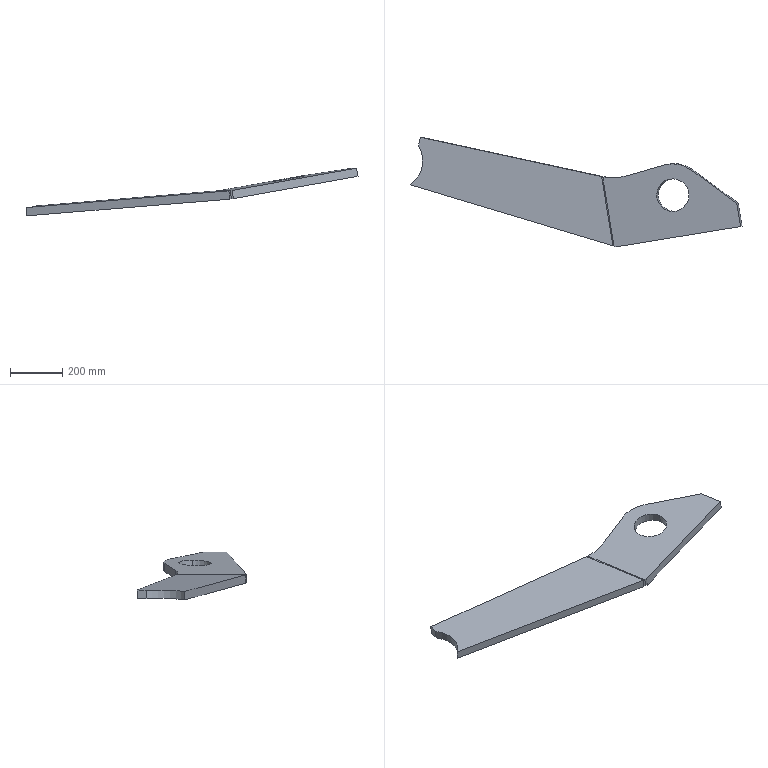Part | SolidWorks | features Cut 1, DeleteBody 1, MirrorSolid 1, SplitBody 1 | 1 solid | 28 faces | box 1270 x 419.262 x 182.493 mm | volume 8566832 mm3 | plane 14 | cylinder 12 | spline 2 | commonest cylinder face diameters 14 x4 125 x2 400 x2 100 x1 164 x1 220 x1
STEP:
#1=CARTESIAN_POINT('',(4240.325,221.645,-697.388));
#2=VERTEX_POINT('',#1);
#3=CARTESIAN_POINT('',(4226.533,221.679,-699.788));
#4=VERTEX_POINT('',#3);
#5=CARTESIAN_POINT('',(4233.429,221.662,-698.588));
#6=DIRECTION('',(-0.1714,-0.02782,0.9848));
#7=DIRECTION('',(0.9852,-0.002402,0.1714));
#8=AXIS2_PLACEMENT_3D('',#5,#6,#7);
#9=CIRCLE('',#8,7.);
#10=EDGE_CURVE('',#2,#4,#9,.T.);
#11=ORIENTED_EDGE('',*,*,#10,.T.);
#12=CARTESIAN_POINT('',(4229.961,222.235,-719.484));
#13=VERTEX_POINT('',#12);
#14=CARTESIAN_POINT('',(4226.533,221.679,-699.788));
#15=DIRECTION('',(0.1714,0.02782,-0.9848));
#16=VECTOR('',#15,1000.);
#17=LINE('',#14,#16);
#18=EDGE_CURVE('',#4,#13,#17,.T.);
#19=ORIENTED_EDGE('',*,*,#18,.T.);
#20=CARTESIAN_POINT('',(4243.754,222.201,-717.084));
#21=VERTEX_POINT('',#20);
#22=CARTESIAN_POINT('',(4236.857,222.218,-718.284));
#23=DIRECTION('',(-0.1714,-0.02782,0.9848));
#24=DIRECTION('',(0.9852,-0.002402,0.1714));
#25=AXIS2_PLACEMENT_3D('',#22,#23,#24);
#26=CIRCLE('',#25,7.);
#27=EDGE_CURVE('',#21,#13,#26,.T.);
#28=ORIENTED_EDGE('',*,*,#27,.F.);
#29=CARTESIAN_POINT('',(4240.325,221.645,-697.388));
#30=DIRECTION('',(0.1714,0.02782,-0.9848));
#31=VECTOR('',#30,1000.);
#32=LINE('',#29,#31);
#33=EDGE_CURVE('',#2,#21,#32,.T.);
#34=ORIENTED_EDGE('',*,*,#33,.F.);
#35=EDGE_LOOP('',(#11,#19,#28,#34));
#36=FACE_OUTER_BOUND('',#35,.T.);
#37=CARTESIAN_POINT('',(4233.429,221.662,-698.588));
#38=DIRECTION('',(0.1714,0.02782,-0.9848));
#39=DIRECTION('',(0.9852,-0.002402,0.1714));
#40=AXIS2_PLACEMENT_3D('',#37,#38,#39);
#41=CYLINDRICAL_SURFACE('',#40,7.);
#42=ADVANCED_FACE('',(#36),#41,.F.);
#43=CARTESIAN_POINT('',(4162.558,209.024,-711.28));
#44=VERTEX_POINT('',#43);
#45=CARTESIAN_POINT('',(4148.766,209.058,-713.679));
#46=VERTEX_POINT('',#45);
#47=CARTESIAN_POINT('',(4155.662,209.041,-712.48));
#48=DIRECTION('',(-0.1714,-0.02782,0.9848));
#49=DIRECTION('',(-0.9852,0.002402,-0.1714));
#50=AXIS2_PLACEMENT_3D('',#47,#48,#49);
#51=CIRCLE('',#50,7.);
#52=EDGE_CURVE('',#44,#46,#51,.T.);
#53=ORIENTED_EDGE('',*,*,#52,.T.);
#54=CARTESIAN_POINT('',(4152.194,209.614,-733.376));
#55=VERTEX_POINT('',#54);
#56=CARTESIAN_POINT('',(4148.766,209.058,-713.679));
#57=DIRECTION('',(0.1714,0.02782,-0.9848));
#58=VECTOR('',#57,1000.);
#59=LINE('',#56,#58);
#60=EDGE_CURVE('',#46,#55,#59,.T.);
#61=ORIENTED_EDGE('',*,*,#60,.T.);
#62=CARTESIAN_POINT('',(4165.986,209.58,-730.976));
#63=VERTEX_POINT('',#62);
#64=CARTESIAN_POINT('',(4159.09,209.597,-732.176));
#65=DIRECTION('',(-0.1714,-0.02782,0.9848));
#66=DIRECTION('',(-0.9852,0.002402,-0.1714));
#67=AXIS2_PLACEMENT_3D('',#64,#65,#66);
#68=CIRCLE('',#67,7.);
#69=EDGE_CURVE('',#63,#55,#68,.T.);
#70=ORIENTED_EDGE('',*,*,#69,.F.);
#71=CARTESIAN_POINT('',(4162.558,209.024,-711.28));
#72=DIRECTION('',(0.1714,0.02782,-0.9848));
#73=VECTOR('',#72,1000.);
#74=LINE('',#71,#73);
#75=EDGE_CURVE('',#44,#63,#74,.T.);
#76=ORIENTED_EDGE('',*,*,#75,.F.);
#77=EDGE_LOOP('',(#53,#61,#70,#76));
#78=FACE_OUTER_BOUND('',#77,.T.);
#79=CARTESIAN_POINT('',(4155.662,209.041,-712.48));
#80=DIRECTION('',(0.1714,0.02782,-0.9848));
#81=DIRECTION('',(0.9852,-0.002402,0.1714));
#82=AXIS2_PLACEMENT_3D('',#79,#80,#81);
#83=CYLINDRICAL_SURFACE('',#82,7.);
#84=ADVANCED_FACE('',(#78),#83,.F.);
#85=CARTESIAN_POINT('',(4126.275,273.475,-736.083));
#86=VERTEX_POINT('',#85);
#87=CARTESIAN_POINT('',(4247.786,293.196,-714.377));
#88=VERTEX_POINT('',#87);
#89=CARTESIAN_POINT('',(4187.031,283.335,-725.23));
#90=DIRECTION('',(0.1714,0.02782,-0.9848));
#91=DIRECTION('',(-0.9721,-0.1578,-0.1736));
#92=AXIS2_PLACEMENT_3D('',#89,#90,#91);
#93=CIRCLE('',#92,62.5);
#94=EDGE_CURVE('',#86,#88,#93,.T.);
#95=ORIENTED_EDGE('',*,*,#94,.T.);
#96=CARTESIAN_POINT('',(4242.301,292.305,-682.863));
#97=VERTEX_POINT('',#96);
#98=CARTESIAN_POINT('',(4247.786,293.196,-714.377));
#99=DIRECTION('',(-0.1714,-0.02782,0.9848));
#100=VECTOR('',#99,1000.);
#101=LINE('',#98,#100);
#102=EDGE_CURVE('',#88,#97,#101,.T.);
#103=ORIENTED_EDGE('',*,*,#102,.T.);
#104=CARTESIAN_POINT('',(4120.79,272.585,-704.569));
#105=VERTEX_POINT('',#104);
#106=CARTESIAN_POINT('',(4181.546,282.445,-693.716));
#107=DIRECTION('',(0.1714,0.02782,-0.9848));
#108=DIRECTION('',(-0.9721,-0.1578,-0.1736));
#109=AXIS2_PLACEMENT_3D('',#106,#107,#108);
#110=CIRCLE('',#109,62.5);
#111=EDGE_CURVE('',#105,#97,#110,.T.);
#112=ORIENTED_EDGE('',*,*,#111,.F.);
#113=CARTESIAN_POINT('',(4126.275,273.475,-736.083));
#114=DIRECTION('',(-0.1714,-0.02782,0.9848));
#115=VECTOR('',#114,1000.);
#116=LINE('',#113,#115);
#117=EDGE_CURVE('',#86,#105,#116,.T.);
#118=ORIENTED_EDGE('',*,*,#117,.F.);
#119=EDGE_LOOP('',(#95,#103,#112,#118));
#120=FACE_OUTER_BOUND('',#119,.T.);
#121=CARTESIAN_POINT('',(4187.031,283.335,-725.23));
#122=DIRECTION('',(-0.1714,-0.02782,0.9848));
#123=DIRECTION('',(-0.9721,-0.1578,-0.1736));
#124=AXIS2_PLACEMENT_3D('',#121,#122,#123);
#125=CYLINDRICAL_SURFACE('',#124,62.5);
#126=ADVANCED_FACE('',(#120),#125,.F.);
#127=ORIENTED_EDGE('',*,*,#27,.T.);
#128=CARTESIAN_POINT('',(4236.857,222.218,-718.284));
#129=DIRECTION('',(-0.1714,-0.02782,0.9848));
#130=DIRECTION('',(0.9852,-0.002402,0.1714));
#131=AXIS2_PLACEMENT_3D('',#128,#129,#130);
#132=CIRCLE('',#131,7.);
#133=EDGE_CURVE('',#13,#21,#132,.T.);
#134=ORIENTED_EDGE('',*,*,#133,.T.);
#135=EDGE_LOOP('',(#127,#134));
#136=FACE_BOUND('',#135,.T.);
#137=ORIENTED_EDGE('',*,*,#69,.T.);
#138=CARTESIAN_POINT('',(4159.09,209.597,-732.176));
#139=DIRECTION('',(-0.1714,-0.02782,0.9848));
#140=DIRECTION('',(-0.9852,0.002402,-0.1714));
#141=AXIS2_PLACEMENT_3D('',#138,#139,#140);
#142=CIRCLE('',#141,7.);
#143=EDGE_CURVE('',#55,#63,#142,.T.);
#144=ORIENTED_EDGE('',*,*,#143,.T.);
#145=EDGE_LOOP('',(#137,#144));
#146=FACE_BOUND('',#145,.T.);
#147=CARTESIAN_POINT('',(4154.416,398.793,-727.645));
#148=VERTEX_POINT('',#147);
#149=CARTESIAN_POINT('',(4255.831,380.546,-710.509));
#150=VERTEX_POINT('',#149);
#151=CARTESIAN_POINT('',(4187.031,283.335,-725.23));
#152=DIRECTION('',(0.1714,0.02782,-0.9848));
#153=DIRECTION('',(-0.9721,-0.1578,-0.1736));
#154=AXIS2_PLACEMENT_3D('',#151,#152,#153);
#155=CIRCLE('',#154,120.);
#156=EDGE_CURVE('',#148,#150,#155,.T.);
#157=ORIENTED_EDGE('',*,*,#156,.T.);
#158=CARTESIAN_POINT('',(4431.546,252.102,-683.554));
#159=VERTEX_POINT('',#158);
#160=CARTESIAN_POINT('',(4431.546,252.102,-683.554));
#161=DIRECTION('',(-0.8012,0.5857,-0.1229));
#162=VECTOR('',#161,1000.);
#163=LINE('',#160,#162);
#164=EDGE_CURVE('',#159,#150,#163,.T.);
#165=ORIENTED_EDGE('',*,*,#164,.F.);
#166=CARTESIAN_POINT('',(4445.963,163.265,-683.554));
#167=VERTEX_POINT('',#166);
#168=CARTESIAN_POINT('',(4445.963,163.265,-683.554));
#169=DIRECTION('',(-0.1602,0.9871,0.));
#170=VECTOR('',#169,1000.);
#171=LINE('',#168,#170);
#172=EDGE_CURVE('',#167,#159,#171,.T.);
#173=ORIENTED_EDGE('',*,*,#172,.F.);
#174=CARTESIAN_POINT('',(3969.64,85.961,-768.642));
#175=VERTEX_POINT('',#174);
#176=CARTESIAN_POINT('',(3969.64,85.961,-768.642));
#177=DIRECTION('',(0.9721,0.1578,0.1736));
#178=VECTOR('',#177,1000.);
#179=LINE('',#176,#178);
#180=EDGE_CURVE('',#175,#167,#179,.T.);
#181=ORIENTED_EDGE('',*,*,#180,.F.);
#182=CARTESIAN_POINT('',(3962.166,88.239,-769.878));
#183=VERTEX_POINT('',#182);
#184=CARTESIAN_POINT('',(3962.166,88.239,-769.878));
#185=DIRECTION('',(0.9448,-0.288,0.1563));
#186=VECTOR('',#185,1000.);
#187=LINE('',#184,#186);
#188=EDGE_CURVE('',#183,#175,#187,.T.);
#189=ORIENTED_EDGE('',*,*,#188,.F.);
#190=CARTESIAN_POINT('',(3919.209,352.929,-769.878));
#191=VERTEX_POINT('',#190);
#192=CARTESIAN_POINT('',(3983.906,-45.716,-769.878));
#193=DIRECTION('',(-0.1602,0.9871,0.));
#194=VECTOR('',#193,1000.);
#195=LINE('',#192,#194);
#196=EDGE_CURVE('',#183,#191,#195,.T.);
#197=ORIENTED_EDGE('',*,*,#196,.T.);
#198=CARTESIAN_POINT('',(4008.632,357.057,-754.198));
#199=VERTEX_POINT('',#198);
#200=CARTESIAN_POINT('',(3954.275,549.486,-758.223));
#201=DIRECTION('',(0.1714,0.02782,-0.9848));
#202=DIRECTION('',(-0.9721,-0.1578,-0.1736));
#203=AXIS2_PLACEMENT_3D('',#200,#201,#202);
#204=CIRCLE('',#203,200.);
#205=EDGE_CURVE('',#199,#191,#204,.T.);
#206=ORIENTED_EDGE('',*,*,#205,.F.);
#207=CARTESIAN_POINT('',(4154.416,398.793,-727.645));
#208=DIRECTION('',(-0.947,-0.2711,-0.1725));
#209=VECTOR('',#208,1000.);
#210=LINE('',#207,#209);
#211=EDGE_CURVE('',#148,#199,#210,.T.);
#212=ORIENTED_EDGE('',*,*,#211,.F.);
#213=EDGE_LOOP('',(#157,#165,#173,#181,#189,#197,#206,#212));
#214=FACE_OUTER_BOUND('',#213,.T.);
#215=ORIENTED_EDGE('',*,*,#94,.F.);
#216=CARTESIAN_POINT('',(4187.031,283.335,-725.23));
#217=DIRECTION('',(0.1714,0.02782,-0.9848));
#218=DIRECTION('',(-0.9721,-0.1578,-0.1736));
#219=AXIS2_PLACEMENT_3D('',#216,#217,#218);
#220=CIRCLE('',#219,62.5);
#221=EDGE_CURVE('',#88,#86,#220,.T.);
#222=ORIENTED_EDGE('',*,*,#221,.F.);
#223=EDGE_LOOP('',(#215,#222));
#224=FACE_BOUND('',#223,.T.);
#225=CARTESIAN_POINT('',(3127.999,415.387,-905.824));
#226=DIRECTION('',(0.1714,0.02782,-0.9848));
#227=DIRECTION('',(0.9721,0.1578,0.1736));
#228=AXIS2_PLACEMENT_3D('',#225,#226,#227);
#229=PLANE('',#228);
#230=ADVANCED_FACE('',(#136,#146,#214,#224),#229,.T.);
#231=CARTESIAN_POINT('',(3956.681,87.349,-738.364));
#232=VERTEX_POINT('',#231);
#233=CARTESIAN_POINT('',(3964.155,85.071,-737.128));
#234=VERTEX_POINT('',#233);
#235=CARTESIAN_POINT('',(3956.681,87.349,-738.364));
#236=DIRECTION('',(0.9448,-0.288,0.1563));
#237=VECTOR('',#236,1000.);
#238=LINE('',#235,#237);
#239=EDGE_CURVE('',#232,#234,#238,.T.);
#240=ORIENTED_EDGE('',*,*,#239,.F.);
#241=CARTESIAN_POINT('',(3959.424,87.794,-754.121));
#242=DIRECTION('',(0.1714,0.02782,-0.9848));
#243=VECTOR('',#242,1000.);
#244=LINE('',#241,#243);
#245=EDGE_CURVE('',#232,#183,#244,.T.);
#246=ORIENTED_EDGE('',*,*,#245,.T.);
#247=ORIENTED_EDGE('',*,*,#188,.T.);
#248=CARTESIAN_POINT('',(3964.155,85.071,-737.128));
#249=DIRECTION('',(0.1714,0.02782,-0.9848));
#250=VECTOR('',#249,1000.);
#251=LINE('',#248,#250);
#252=EDGE_CURVE('',#234,#175,#251,.T.);
#253=ORIENTED_EDGE('',*,*,#252,.F.);
#254=EDGE_LOOP('',(#240,#246,#247,#253));
#255=FACE_OUTER_BOUND('',#254,.T.);
#256=CARTESIAN_POINT('',(3188.722,324.015,-897.836));
#257=DIRECTION('',(0.2793,0.9572,0.07565));
#258=DIRECTION('',(-0.9553,0.2849,-0.07851));
#259=AXIS2_PLACEMENT_3D('',#256,#257,#258);
#260=PLANE('',#259);
#261=ADVANCED_FACE('',(#255),#260,.F.);
#262=CARTESIAN_POINT('',(4440.478,162.375,-652.04));
#263=VERTEX_POINT('',#262);
#264=CARTESIAN_POINT('',(4445.963,163.265,-683.554));
#265=DIRECTION('',(0.1714,0.02782,-0.9848));
#266=VECTOR('',#265,1000.);
#267=LINE('',#264,#266);
#268=EDGE_CURVE('',#263,#167,#267,.T.);
#269=ORIENTED_EDGE('',*,*,#268,.F.);
#270=CARTESIAN_POINT('',(3196.204,-39.562,-874.31));
#271=DIRECTION('',(0.9721,0.1578,0.1736));
#272=VECTOR('',#271,1000.);
#273=LINE('',#270,#272);
#274=EDGE_CURVE('',#234,#263,#273,.T.);
#275=ORIENTED_EDGE('',*,*,#274,.F.);
#276=ORIENTED_EDGE('',*,*,#252,.T.);
#277=ORIENTED_EDGE('',*,*,#180,.T.);
#278=EDGE_LOOP('',(#269,#275,#276,#277));
#279=FACE_OUTER_BOUND('',#278,.T.);
#280=CARTESIAN_POINT('',(3969.64,85.961,-768.642));
#281=DIRECTION('',(-0.1602,0.9871,0.));
#282=DIRECTION('',(0.08603,0.01396,-0.9962));
#283=AXIS2_PLACEMENT_3D('',#280,#281,#282);
#284=PLANE('',#283);
#285=ADVANCED_FACE('',(#279),#284,.F.);
#286=CARTESIAN_POINT('',(4426.061,251.212,-652.04));
#287=VERTEX_POINT('',#286);
#288=CARTESIAN_POINT('',(4426.061,251.212,-652.04));
#289=DIRECTION('',(0.1714,0.02782,-0.9848));
#290=VECTOR('',#289,1000.);
#291=LINE('',#288,#290);
#292=EDGE_CURVE('',#287,#159,#291,.T.);
#293=ORIENTED_EDGE('',*,*,#292,.F.);
#294=CARTESIAN_POINT('',(4366.788,616.434,-652.04));
#295=DIRECTION('',(-0.1602,0.9871,0.));
#296=VECTOR('',#295,1000.);
#297=LINE('',#294,#296);
#298=EDGE_CURVE('',#263,#287,#297,.T.);
#299=ORIENTED_EDGE('',*,*,#298,.F.);
#300=ORIENTED_EDGE('',*,*,#268,.T.);
#301=ORIENTED_EDGE('',*,*,#172,.T.);
#302=EDGE_LOOP('',(#293,#299,#300,#301));
#303=FACE_OUTER_BOUND('',#302,.T.);
#304=CARTESIAN_POINT('',(4445.963,163.265,-683.554));
#305=DIRECTION('',(-0.9721,-0.1578,-0.1736));
#306=DIRECTION('',(0.1714,0.02782,-0.9848));
#307=AXIS2_PLACEMENT_3D('',#304,#305,#306);
#308=PLANE('',#307);
#309=ADVANCED_FACE('',(#303),#308,.F.);
#310=CARTESIAN_POINT('',(4250.346,379.656,-678.995));
#311=VERTEX_POINT('',#310);
#312=CARTESIAN_POINT('',(4255.831,380.546,-710.509));
#313=DIRECTION('',(-0.1714,-0.02782,0.9848));
#314=VECTOR('',#313,1000.);
#315=LINE('',#312,#314);
#316=EDGE_CURVE('',#150,#311,#315,.T.);
#317=ORIENTED_EDGE('',*,*,#316,.T.);
#318=CARTESIAN_POINT('',(4426.061,251.212,-652.04));
#319=DIRECTION('',(-0.8012,0.5857,-0.1229));
#320=VECTOR('',#319,1000.);
#321=LINE('',#318,#320);
#322=EDGE_CURVE('',#287,#311,#321,.T.);
#323=ORIENTED_EDGE('',*,*,#322,.F.);
#324=ORIENTED_EDGE('',*,*,#292,.T.);
#325=ORIENTED_EDGE('',*,*,#164,.T.);
#326=EDGE_LOOP('',(#317,#323,#324,#325));
#327=FACE_OUTER_BOUND('',#326,.T.);
#328=CARTESIAN_POINT('',(4431.546,252.102,-683.554));
#329=DIRECTION('',(-0.5733,-0.8101,-0.1227));
#330=DIRECTION('',(0.8103,-0.5828,0.0618));
#331=AXIS2_PLACEMENT_3D('',#328,#329,#330);
#332=PLANE('',#331);
#333=ADVANCED_FACE('',(#327),#332,.F.);
#334=ORIENTED_EDGE('',*,*,#156,.F.);
#335=CARTESIAN_POINT('',(4148.931,397.903,-696.131));
#336=VERTEX_POINT('',#335);
#337=CARTESIAN_POINT('',(4148.931,397.903,-696.131));
#338=DIRECTION('',(0.1714,0.02782,-0.9848));
#339=VECTOR('',#338,1000.);
#340=LINE('',#337,#339);
#341=EDGE_CURVE('',#336,#148,#340,.T.);
#342=ORIENTED_EDGE('',*,*,#341,.F.);
#343=CARTESIAN_POINT('',(4181.546,282.445,-693.716));
#344=DIRECTION('',(-0.1714,-0.02782,0.9848));
#345=DIRECTION('',(-0.9721,-0.1578,-0.1736));
#346=AXIS2_PLACEMENT_3D('',#343,#344,#345);
#347=CIRCLE('',#346,120.);
#348=EDGE_CURVE('',#311,#336,#347,.T.);
#349=ORIENTED_EDGE('',*,*,#348,.F.);
#350=ORIENTED_EDGE('',*,*,#316,.F.);
#351=EDGE_LOOP('',(#334,#342,#349,#350));
#352=FACE_OUTER_BOUND('',#351,.T.);
#353=CARTESIAN_POINT('',(4187.031,283.335,-725.23));
#354=DIRECTION('',(-0.1714,-0.02782,0.9848));
#355=DIRECTION('',(-0.9721,-0.1578,-0.1736));
#356=AXIS2_PLACEMENT_3D('',#353,#354,#355);
#357=CYLINDRICAL_SURFACE('',#356,120.);
#358=ADVANCED_FACE('',(#352),#357,.T.);
#359=CARTESIAN_POINT('',(4003.147,356.166,-722.684));
#360=VERTEX_POINT('',#359);
#361=CARTESIAN_POINT('',(4008.632,357.057,-754.198));
#362=DIRECTION('',(0.1714,0.02782,-0.9848));
#363=VECTOR('',#362,1000.);
#364=LINE('',#361,#363);
#365=EDGE_CURVE('',#360,#199,#364,.T.);
#366=ORIENTED_EDGE('',*,*,#365,.F.);
#367=CARTESIAN_POINT('',(4148.931,397.903,-696.131));
#368=DIRECTION('',(-0.947,-0.2711,-0.1725));
#369=VECTOR('',#368,1000.);
#370=LINE('',#367,#369);
#371=EDGE_CURVE('',#336,#360,#370,.T.);
#372=ORIENTED_EDGE('',*,*,#371,.F.);
#373=ORIENTED_EDGE('',*,*,#341,.T.);
#374=ORIENTED_EDGE('',*,*,#211,.T.);
#375=EDGE_LOOP('',(#366,#372,#373,#374));
#376=FACE_OUTER_BOUND('',#375,.T.);
#377=CARTESIAN_POINT('',(4154.416,398.793,-727.645));
#378=DIRECTION('',(0.2718,-0.9621,0.02013));
#379=DIRECTION('',(0.9583,0.2725,0.08657));
#380=AXIS2_PLACEMENT_3D('',#377,#378,#379);
#381=PLANE('',#380);
#382=ADVANCED_FACE('',(#376),#381,.F.);
#383=ORIENTED_EDGE('',*,*,#102,.F.);
#384=ORIENTED_EDGE('',*,*,#221,.T.);
#385=ORIENTED_EDGE('',*,*,#117,.T.);
#386=CARTESIAN_POINT('',(4181.546,282.445,-693.716));
#387=DIRECTION('',(0.1714,0.02782,-0.9848));
#388=DIRECTION('',(-0.9721,-0.1578,-0.1736));
#389=AXIS2_PLACEMENT_3D('',#386,#387,#388);
#390=CIRCLE('',#389,62.5);
#391=EDGE_CURVE('',#97,#105,#390,.T.);
#392=ORIENTED_EDGE('',*,*,#391,.F.);
#393=EDGE_LOOP('',(#383,#384,#385,#392));
#394=FACE_OUTER_BOUND('',#393,.T.);
#395=CARTESIAN_POINT('',(4187.031,283.335,-725.23));
#396=DIRECTION('',(-0.1714,-0.02782,0.9848));
#397=DIRECTION('',(-0.9721,-0.1578,-0.1736));
#398=AXIS2_PLACEMENT_3D('',#395,#396,#397);
#399=CYLINDRICAL_SURFACE('',#398,62.5);
#400=ADVANCED_FACE('',(#394),#399,.F.);
#401=ORIENTED_EDGE('',*,*,#205,.T.);
#402=CARTESIAN_POINT('',(3913.724,352.039,-738.364));
#403=VERTEX_POINT('',#402);
#404=CARTESIAN_POINT('',(3916.467,352.484,-754.121));
#405=DIRECTION('',(-0.1714,-0.02782,0.9848));
#406=VECTOR('',#405,1000.);
#407=LINE('',#404,#406);
#408=EDGE_CURVE('',#191,#403,#407,.T.);
#409=ORIENTED_EDGE('',*,*,#408,.T.);
#410=CARTESIAN_POINT('',(3948.79,548.596,-726.709));
#411=DIRECTION('',(0.1714,0.02782,-0.9848));
#412=DIRECTION('',(-0.9721,-0.1578,-0.1736));
#413=AXIS2_PLACEMENT_3D('',#410,#411,#412);
#414=CIRCLE('',#413,200.);
#415=EDGE_CURVE('',#360,#403,#414,.T.);
#416=ORIENTED_EDGE('',*,*,#415,.F.);
#417=ORIENTED_EDGE('',*,*,#365,.T.);
#418=EDGE_LOOP('',(#401,#409,#416,#417));
#419=FACE_OUTER_BOUND('',#418,.T.);
#420=CARTESIAN_POINT('',(3954.275,549.486,-758.223));
#421=DIRECTION('',(-0.1714,-0.02782,0.9848));
#422=DIRECTION('',(-0.9721,-0.1578,-0.1736));
#423=AXIS2_PLACEMENT_3D('',#420,#421,#422);
#424=CYLINDRICAL_SURFACE('',#423,200.);
#425=ADVANCED_FACE('',(#419),#424,.F.);
#426=ORIENTED_EDGE('',*,*,#196,.F.);
#427=CARTESIAN_POINT('',(3954.719,89.855,-770.812));
#428=VERTEX_POINT('',#427);
#429=CARTESIAN_POINT('',(3962.166,88.239,-769.878));
#430=CARTESIAN_POINT('',(3959.699,88.78,-770.293));
#431=CARTESIAN_POINT('',(3957.213,89.318,-770.604));
#432=CARTESIAN_POINT('',(3954.719,89.855,-770.812));
#433=B_SPLINE_CURVE_WITH_KNOTS('',3,(#429,#430,#431,#432),.UNSPECIFIED.,.F.,.F.,(4,4),(0.,1.),.UNSPECIFIED.);
#434=EDGE_CURVE('',#183,#428,#433,.T.);
#435=ORIENTED_EDGE('',*,*,#434,.T.);
#436=CARTESIAN_POINT('',(3911.863,353.917,-770.812));
#437=VERTEX_POINT('',#436);
#438=CARTESIAN_POINT('',(3882.027,537.761,-770.812));
#439=DIRECTION('',(-0.1602,0.9871,0.));
#440=VECTOR('',#439,1000.);
#441=LINE('',#438,#440);
#442=EDGE_CURVE('',#428,#437,#441,.T.);
#443=ORIENTED_EDGE('',*,*,#442,.T.);
#444=CARTESIAN_POINT('',(3911.863,353.917,-770.812));
#445=CARTESIAN_POINT('',(3914.324,353.59,-770.604));
#446=CARTESIAN_POINT('',(3916.775,353.261,-770.293));
#447=CARTESIAN_POINT('',(3919.209,352.929,-769.878));
#448=B_SPLINE_CURVE_WITH_KNOTS('',3,(#444,#445,#446,#447),.UNSPECIFIED.,.F.,.F.,(4,4),(0.,1.),.UNSPECIFIED.);
#449=EDGE_CURVE('',#437,#191,#448,.T.);
#450=ORIENTED_EDGE('',*,*,#449,.T.);
#451=EDGE_LOOP('',(#426,#435,#443,#450));
#452=FACE_OUTER_BOUND('',#451,.T.);
#453=CARTESIAN_POINT('',(3969.851,-47.997,-689.124));
#454=DIRECTION('',(-0.1602,0.9871,0.));
#455=DIRECTION('',(0.08603,0.01396,-0.9962));
#456=AXIS2_PLACEMENT_3D('',#453,#454,#455);
#457=CYLINDRICAL_SURFACE('',#456,82.);
#458=ADVANCED_FACE('',(#452),#457,.T.);
#459=CARTESIAN_POINT('',(3909.11,353.471,-738.934));
#460=VERTEX_POINT('',#459);
#461=CARTESIAN_POINT('',(3910.487,353.694,-754.873));
#462=DIRECTION('',(0.08603,0.01396,-0.9962));
#463=VECTOR('',#462,1000.);
#464=LINE('',#461,#463);
#465=EDGE_CURVE('',#460,#437,#464,.T.);
#466=ORIENTED_EDGE('',*,*,#465,.T.);
#467=CARTESIAN_POINT('',(3911.799,353.931,-770.817));
#468=VERTEX_POINT('',#467);
#469=CARTESIAN_POINT('',(3911.863,353.917,-770.812));
#470=DIRECTION('',(-0.9741,0.2112,-0.08116));
#471=VECTOR('',#470,1000.);
#472=LINE('',#469,#471);
#473=EDGE_CURVE('',#437,#468,#472,.T.);
#474=ORIENTED_EDGE('',*,*,#473,.T.);
#475=CARTESIAN_POINT('',(3909.046,353.485,-738.939));
#476=VERTEX_POINT('',#475);
#477=CARTESIAN_POINT('',(3911.799,353.931,-770.817));
#478=DIRECTION('',(0.08603,0.01396,-0.9962));
#479=VECTOR('',#478,1000.);
#480=LINE('',#477,#479);
#481=EDGE_CURVE('',#476,#468,#480,.T.);
#482=ORIENTED_EDGE('',*,*,#481,.F.);
#483=CARTESIAN_POINT('',(3950.939,548.945,-732.582));
#484=DIRECTION('',(-0.08603,-0.01396,0.9962));
#485=DIRECTION('',(-0.9833,-0.1596,-0.08716));
#486=AXIS2_PLACEMENT_3D('',#483,#484,#485);
#487=CIRCLE('',#486,200.);
#488=EDGE_CURVE('',#476,#460,#487,.T.);
#489=ORIENTED_EDGE('',*,*,#488,.T.);
#490=EDGE_LOOP('',(#466,#474,#482,#489));
#491=FACE_OUTER_BOUND('',#490,.T.);
#492=CARTESIAN_POINT('',(3953.692,549.391,-764.46));
#493=DIRECTION('',(-0.08603,-0.01396,0.9962));
#494=DIRECTION('',(-0.9833,-0.1596,-0.08716));
#495=AXIS2_PLACEMENT_3D('',#492,#493,#494);
#496=CYLINDRICAL_SURFACE('',#495,200.);
#497=ADVANCED_FACE('',(#491),#496,.F.);
#498=CARTESIAN_POINT('',(3211.598,470.615,-829.651));
#499=VERTEX_POINT('',#498);
#500=CARTESIAN_POINT('',(3179.102,322.454,-834.533));
#501=VERTEX_POINT('',#500);
#502=CARTESIAN_POINT('',(3117.862,413.742,-838.543));
#503=DIRECTION('',(0.08603,0.01396,-0.9962));
#504=DIRECTION('',(-0.9833,-0.1596,-0.08716));
#505=AXIS2_PLACEMENT_3D('',#502,#503,#504);
#506=CIRCLE('',#505,110.);
#507=EDGE_CURVE('',#499,#501,#506,.T.);
#508=ORIENTED_EDGE('',*,*,#507,.F.);
#509=CARTESIAN_POINT('',(3218.825,504.333,-828.554));
#510=VERTEX_POINT('',#509);
#511=CARTESIAN_POINT('',(3218.825,504.333,-828.554));
#512=DIRECTION('',(-0.2095,-0.9773,-0.03179));
#513=VECTOR('',#512,1000.);
#514=LINE('',#511,#513);
#515=EDGE_CURVE('',#510,#499,#514,.T.);
#516=ORIENTED_EDGE('',*,*,#515,.F.);
#517=CARTESIAN_POINT('',(3218.825,504.333,-828.554));
#518=DIRECTION('',(-0.974,0.2114,-0.08115));
#519=VECTOR('',#518,1000.);
#520=LINE('',#517,#519);
#521=EDGE_CURVE('',#468,#510,#520,.T.);
#522=ORIENTED_EDGE('',*,*,#521,.F.);
#523=ORIENTED_EDGE('',*,*,#473,.F.);
#524=ORIENTED_EDGE('',*,*,#442,.F.);
#525=CARTESIAN_POINT('',(3179.102,322.454,-834.533));
#526=DIRECTION('',(0.9549,-0.2864,0.07845));
#527=VECTOR('',#526,1000.);
#528=LINE('',#525,#527);
#529=EDGE_CURVE('',#501,#428,#528,.T.);
#530=ORIENTED_EDGE('',*,*,#529,.F.);
#531=EDGE_LOOP('',(#508,#516,#522,#523,#524,#530));
#532=FACE_OUTER_BOUND('',#531,.T.);
#533=CARTESIAN_POINT('',(3117.862,413.742,-838.543));
#534=DIRECTION('',(0.08603,0.01396,-0.9962));
#535=DIRECTION('',(0.9833,0.1596,0.08716));
#536=AXIS2_PLACEMENT_3D('',#533,#534,#535);
#537=PLANE('',#536);
#538=ADVANCED_FACE('',(#532),#537,.T.);
#539=ORIENTED_EDGE('',*,*,#434,.F.);
#540=ORIENTED_EDGE('',*,*,#245,.F.);
#541=CARTESIAN_POINT('',(3951.966,89.408,-738.934));
#542=VERTEX_POINT('',#541);
#543=CARTESIAN_POINT('',(3951.966,89.408,-738.934));
#544=CARTESIAN_POINT('',(3953.545,88.723,-738.807));
#545=CARTESIAN_POINT('',(3955.119,88.037,-738.617));
#546=CARTESIAN_POINT('',(3956.681,87.349,-738.364));
#547=B_SPLINE_CURVE_WITH_KNOTS('',3,(#543,#544,#545,#546),.UNSPECIFIED.,.F.,.F.,(4,4),(0.,1.),.UNSPECIFIED.);
#548=EDGE_CURVE('',#542,#232,#547,.T.);
#549=ORIENTED_EDGE('',*,*,#548,.F.);
#550=CARTESIAN_POINT('',(3954.719,89.855,-770.812));
#551=DIRECTION('',(-0.08603,-0.01396,0.9962));
#552=VECTOR('',#551,1000.);
#553=LINE('',#550,#552);
#554=EDGE_CURVE('',#428,#542,#553,.T.);
#555=ORIENTED_EDGE('',*,*,#554,.F.);
#556=EDGE_LOOP('',(#539,#540,#549,#555));
#557=FACE_OUTER_BOUND('',#556,.T.);
#558=CARTESIAN_POINT('',(3954.746,89.859,-771.131));
#559=CARTESIAN_POINT('',(3957.25,89.324,-770.922));
#560=CARTESIAN_POINT('',(3959.744,88.788,-770.609));
#561=CARTESIAN_POINT('',(3962.221,88.248,-770.193));
#562=CARTESIAN_POINT('',(3954.719,89.855,-770.812));
#563=CARTESIAN_POINT('',(3957.213,89.318,-770.604));
#564=CARTESIAN_POINT('',(3959.699,88.78,-770.293));
#565=CARTESIAN_POINT('',(3962.166,88.239,-769.878));
#566=CARTESIAN_POINT('',(3951.966,89.408,-738.934));
#567=CARTESIAN_POINT('',(3953.545,88.723,-738.807));
#568=CARTESIAN_POINT('',(3955.119,88.037,-738.617));
#569=CARTESIAN_POINT('',(3956.681,87.349,-738.364));
#570=B_SPLINE_SURFACE_WITH_KNOTS('',1,3,((#558,#559,#560,#561),(#562,#563,#564,#565),(#566,#567,#568,#569)),.UNSPECIFIED.,.F.,.F.,.F.,(2,1,2),(4,4),(-0.01,0.,1.),(0.,1.),.UNSPECIFIED.);
#571=ADVANCED_FACE('',(#557),#570,.F.);
#572=ORIENTED_EDGE('',*,*,#111,.T.);
#573=ORIENTED_EDGE('',*,*,#391,.T.);
#574=EDGE_LOOP('',(#572,#573));
#575=FACE_BOUND('',#574,.T.);
#576=ORIENTED_EDGE('',*,*,#415,.T.);
#577=CARTESIAN_POINT('',(3978.421,-46.606,-738.364));
#578=DIRECTION('',(-0.1602,0.9871,0.));
#579=VECTOR('',#578,1000.);
#580=LINE('',#577,#579);
#581=EDGE_CURVE('',#232,#403,#580,.T.);
#582=ORIENTED_EDGE('',*,*,#581,.F.);
#583=ORIENTED_EDGE('',*,*,#239,.T.);
#584=ORIENTED_EDGE('',*,*,#274,.T.);
#585=ORIENTED_EDGE('',*,*,#298,.T.);
#586=ORIENTED_EDGE('',*,*,#322,.T.);
#587=ORIENTED_EDGE('',*,*,#348,.T.);
#588=ORIENTED_EDGE('',*,*,#371,.T.);
#589=EDGE_LOOP('',(#576,#582,#583,#584,#585,#586,#587,#588));
#590=FACE_OUTER_BOUND('',#589,.T.);
#591=CARTESIAN_POINT('',(3122.514,414.497,-874.31));
#592=DIRECTION('',(0.1714,0.02782,-0.9848));
#593=DIRECTION('',(0.9721,0.1578,0.1736));
#594=AXIS2_PLACEMENT_3D('',#591,#592,#593);
#595=PLANE('',#594);
#596=ADVANCED_FACE('',(#575,#590),#595,.F.);
#597=ORIENTED_EDGE('',*,*,#465,.F.);
#598=CARTESIAN_POINT('',(3913.724,352.039,-738.364));
#599=CARTESIAN_POINT('',(3912.195,352.518,-738.617));
#600=CARTESIAN_POINT('',(3910.656,352.995,-738.807));
#601=CARTESIAN_POINT('',(3909.11,353.471,-738.934));
#602=B_SPLINE_CURVE_WITH_KNOTS('',3,(#598,#599,#600,#601),.UNSPECIFIED.,.F.,.F.,(4,4),(0.,1.),.UNSPECIFIED.);
#603=EDGE_CURVE('',#403,#460,#602,.T.);
#604=ORIENTED_EDGE('',*,*,#603,.F.);
#605=ORIENTED_EDGE('',*,*,#408,.F.);
#606=ORIENTED_EDGE('',*,*,#449,.F.);
#607=EDGE_LOOP('',(#597,#604,#605,#606));
#608=FACE_OUTER_BOUND('',#607,.T.);
#609=CARTESIAN_POINT('',(3919.264,352.938,-770.193));
#610=CARTESIAN_POINT('',(3916.821,353.268,-770.609));
#611=CARTESIAN_POINT('',(3914.361,353.596,-770.922));
#612=CARTESIAN_POINT('',(3911.891,353.922,-771.131));
#613=CARTESIAN_POINT('',(3919.209,352.929,-769.878));
#614=CARTESIAN_POINT('',(3916.775,353.261,-770.293));
#615=CARTESIAN_POINT('',(3914.324,353.59,-770.604));
#616=CARTESIAN_POINT('',(3911.863,353.917,-770.812));
#617=CARTESIAN_POINT('',(3913.724,352.039,-738.364));
#618=CARTESIAN_POINT('',(3912.195,352.518,-738.617));
#619=CARTESIAN_POINT('',(3910.656,352.995,-738.807));
#620=CARTESIAN_POINT('',(3909.11,353.471,-738.934));
#621=B_SPLINE_SURFACE_WITH_KNOTS('',1,3,((#609,#610,#611,#612),(#613,#614,#615,#616),(#617,#618,#619,#620)),.UNSPECIFIED.,.F.,.F.,.F.,(2,1,2),(4,4),(-0.01,0.,1.),(0.,1.),.UNSPECIFIED.);
#622=ADVANCED_FACE('',(#608),#621,.F.);
#623=CARTESIAN_POINT('',(3216.072,503.887,-796.676));
#624=VERTEX_POINT('',#623);
#625=CARTESIAN_POINT('',(3218.825,504.333,-828.554));
#626=DIRECTION('',(0.08603,0.01396,-0.9962));
#627=VECTOR('',#626,1000.);
#628=LINE('',#625,#627);
#629=EDGE_CURVE('',#624,#510,#628,.T.);
#630=ORIENTED_EDGE('',*,*,#629,.F.);
#631=CARTESIAN_POINT('',(3909.046,353.485,-738.939));
#632=DIRECTION('',(-0.974,0.2114,-0.08115));
#633=VECTOR('',#632,1000.);
#634=LINE('',#631,#633);
#635=EDGE_CURVE('',#476,#624,#634,.T.);
#636=ORIENTED_EDGE('',*,*,#635,.F.);
#637=ORIENTED_EDGE('',*,*,#481,.T.);
#638=ORIENTED_EDGE('',*,*,#521,.T.);
#639=EDGE_LOOP('',(#630,#636,#637,#638));
#640=FACE_OUTER_BOUND('',#639,.T.);
#641=CARTESIAN_POINT('',(3218.825,504.333,-828.554));
#642=DIRECTION('',(-0.2095,-0.9773,-0.03179));
#643=DIRECTION('',(0.974,-0.2114,0.08115));
#644=AXIS2_PLACEMENT_3D('',#641,#642,#643);
#645=PLANE('',#644);
#646=ADVANCED_FACE('',(#640),#645,.F.);
#647=CARTESIAN_POINT('',(3208.845,470.168,-797.772));
#648=VERTEX_POINT('',#647);
#649=CARTESIAN_POINT('',(3211.598,470.615,-829.651));
#650=DIRECTION('',(0.08603,0.01396,-0.9962));
#651=VECTOR('',#650,1000.);
#652=LINE('',#649,#651);
#653=EDGE_CURVE('',#648,#499,#652,.T.);
#654=ORIENTED_EDGE('',*,*,#653,.F.);
#655=CARTESIAN_POINT('',(3216.072,503.887,-796.676));
#656=DIRECTION('',(-0.2095,-0.9773,-0.03179));
#657=VECTOR('',#656,1000.);
#658=LINE('',#655,#657);
#659=EDGE_CURVE('',#624,#648,#658,.T.);
#660=ORIENTED_EDGE('',*,*,#659,.F.);
#661=ORIENTED_EDGE('',*,*,#629,.T.);
#662=ORIENTED_EDGE('',*,*,#515,.T.);
#663=EDGE_LOOP('',(#654,#660,#661,#662));
#664=FACE_OUTER_BOUND('',#663,.T.);
#665=CARTESIAN_POINT('',(3218.825,504.333,-828.554));
#666=DIRECTION('',(0.974,-0.2114,0.08115));
#667=DIRECTION('',(0.2095,0.9773,0.03179));
#668=AXIS2_PLACEMENT_3D('',#665,#666,#667);
#669=PLANE('',#668);
#670=ADVANCED_FACE('',(#664),#669,.F.);
#671=CARTESIAN_POINT('',(3176.349,322.007,-802.655));
#672=VERTEX_POINT('',#671);
#673=CARTESIAN_POINT('',(3179.102,322.454,-834.533));
#674=DIRECTION('',(0.08603,0.01396,-0.9962));
#675=VECTOR('',#674,1000.);
#676=LINE('',#673,#675);
#677=EDGE_CURVE('',#672,#501,#676,.T.);
#678=ORIENTED_EDGE('',*,*,#677,.F.);
#679=CARTESIAN_POINT('',(3115.109,413.296,-806.664));
#680=DIRECTION('',(0.08603,0.01396,-0.9962));
#681=DIRECTION('',(-0.9833,-0.1596,-0.08716));
#682=AXIS2_PLACEMENT_3D('',#679,#680,#681);
#683=CIRCLE('',#682,110.);
#684=EDGE_CURVE('',#648,#672,#683,.T.);
#685=ORIENTED_EDGE('',*,*,#684,.F.);
#686=ORIENTED_EDGE('',*,*,#653,.T.);
#687=ORIENTED_EDGE('',*,*,#507,.T.);
#688=EDGE_LOOP('',(#678,#685,#686,#687));
#689=FACE_OUTER_BOUND('',#688,.T.);
#690=CARTESIAN_POINT('',(3117.862,413.742,-838.543));
#691=DIRECTION('',(-0.08603,-0.01396,0.9962));
#692=DIRECTION('',(-0.9833,-0.1596,-0.08716));
#693=AXIS2_PLACEMENT_3D('',#690,#691,#692);
#694=CYLINDRICAL_SURFACE('',#693,110.);
#695=ADVANCED_FACE('',(#689),#694,.F.);
#696=ORIENTED_EDGE('',*,*,#554,.T.);
#697=CARTESIAN_POINT('',(3176.349,322.007,-802.655));
#698=DIRECTION('',(0.9549,-0.2864,0.07845));
#699=VECTOR('',#698,1000.);
#700=LINE('',#697,#699);
#701=EDGE_CURVE('',#672,#542,#700,.T.);
#702=ORIENTED_EDGE('',*,*,#701,.F.);
#703=ORIENTED_EDGE('',*,*,#677,.T.);
#704=ORIENTED_EDGE('',*,*,#529,.T.);
#705=EDGE_LOOP('',(#696,#702,#703,#704));
#706=FACE_OUTER_BOUND('',#705,.T.);
#707=CARTESIAN_POINT('',(3179.102,322.454,-834.533));
#708=DIRECTION('',(0.2842,0.958,0.03797));
#709=DIRECTION('',(-0.9549,0.2864,-0.07845));
#710=AXIS2_PLACEMENT_3D('',#707,#708,#709);
#711=PLANE('',#710);
#712=ADVANCED_FACE('',(#706),#711,.F.);
#713=ORIENTED_EDGE('',*,*,#603,.T.);
#714=CARTESIAN_POINT('',(3879.274,537.314,-738.934));
#715=DIRECTION('',(-0.1602,0.9871,0.));
#716=VECTOR('',#715,1000.);
#717=LINE('',#714,#716);
#718=EDGE_CURVE('',#542,#460,#717,.T.);
#719=ORIENTED_EDGE('',*,*,#718,.F.);
#720=ORIENTED_EDGE('',*,*,#548,.T.);
#721=ORIENTED_EDGE('',*,*,#581,.T.);
#722=EDGE_LOOP('',(#713,#719,#720,#721));
#723=FACE_OUTER_BOUND('',#722,.T.);
#724=CARTESIAN_POINT('',(3969.851,-47.997,-689.124));
#725=DIRECTION('',(-0.1602,0.9871,0.));
#726=DIRECTION('',(0.08603,0.01396,-0.9962));
#727=AXIS2_PLACEMENT_3D('',#724,#725,#726);
#728=CYLINDRICAL_SURFACE('',#727,50.);
#729=ADVANCED_FACE('',(#723),#728,.F.);
#730=ORIENTED_EDGE('',*,*,#718,.T.);
#731=ORIENTED_EDGE('',*,*,#488,.F.);
#732=ORIENTED_EDGE('',*,*,#635,.T.);
#733=ORIENTED_EDGE('',*,*,#659,.T.);
#734=ORIENTED_EDGE('',*,*,#684,.T.);
#735=ORIENTED_EDGE('',*,*,#701,.T.);
#736=EDGE_LOOP('',(#730,#731,#732,#733,#734,#735));
#737=FACE_OUTER_BOUND('',#736,.T.);
#738=CARTESIAN_POINT('',(3115.109,413.296,-806.664));
#739=DIRECTION('',(0.08603,0.01396,-0.9962));
#740=DIRECTION('',(0.9833,0.1596,0.08716));
#741=AXIS2_PLACEMENT_3D('',#738,#739,#740);
#742=PLANE('',#741);
#743=ADVANCED_FACE('',(#737),#742,.F.);
#744=ORIENTED_EDGE('',*,*,#60,.F.);
#745=CARTESIAN_POINT('',(4155.662,209.041,-712.48));
#746=DIRECTION('',(-0.1714,-0.02782,0.9848));
#747=DIRECTION('',(-0.9852,0.002402,-0.1714));
#748=AXIS2_PLACEMENT_3D('',#745,#746,#747);
#749=CIRCLE('',#748,7.);
#750=EDGE_CURVE('',#46,#44,#749,.T.);
#751=ORIENTED_EDGE('',*,*,#750,.T.);
#752=ORIENTED_EDGE('',*,*,#75,.T.);
#753=ORIENTED_EDGE('',*,*,#143,.F.);
#754=EDGE_LOOP('',(#744,#751,#752,#753));
#755=FACE_OUTER_BOUND('',#754,.T.);
#756=CARTESIAN_POINT('',(4155.662,209.041,-712.48));
#757=DIRECTION('',(0.1714,0.02782,-0.9848));
#758=DIRECTION('',(0.9852,-0.002402,0.1714));
#759=AXIS2_PLACEMENT_3D('',#756,#757,#758);
#760=CYLINDRICAL_SURFACE('',#759,7.);
#761=ADVANCED_FACE('',(#755),#760,.F.);
#762=ORIENTED_EDGE('',*,*,#52,.F.);
#763=ORIENTED_EDGE('',*,*,#750,.F.);
#764=EDGE_LOOP('',(#762,#763));
#765=FACE_OUTER_BOUND('',#764,.T.);
#766=CARTESIAN_POINT('',(4155.662,209.041,-712.48));
#767=DIRECTION('',(-0.1714,-0.02782,0.9848));
#768=DIRECTION('',(-0.9852,0.002402,-0.1714));
#769=AXIS2_PLACEMENT_3D('',#766,#767,#768);
#770=PLANE('',#769);
#771=ADVANCED_FACE('',(#765),#770,.F.);
#772=ORIENTED_EDGE('',*,*,#18,.F.);
#773=CARTESIAN_POINT('',(4233.429,221.662,-698.588));
#774=DIRECTION('',(-0.1714,-0.02782,0.9848));
#775=DIRECTION('',(0.9852,-0.002402,0.1714));
#776=AXIS2_PLACEMENT_3D('',#773,#774,#775);
#777=CIRCLE('',#776,7.);
#778=EDGE_CURVE('',#4,#2,#777,.T.);
#779=ORIENTED_EDGE('',*,*,#778,.T.);
#780=ORIENTED_EDGE('',*,*,#33,.T.);
#781=ORIENTED_EDGE('',*,*,#133,.F.);
#782=EDGE_LOOP('',(#772,#779,#780,#781));
#783=FACE_OUTER_BOUND('',#782,.T.);
#784=CARTESIAN_POINT('',(4233.429,221.662,-698.588));
#785=DIRECTION('',(0.1714,0.02782,-0.9848));
#786=DIRECTION('',(0.9852,-0.002402,0.1714));
#787=AXIS2_PLACEMENT_3D('',#784,#785,#786);
#788=CYLINDRICAL_SURFACE('',#787,7.);
#789=ADVANCED_FACE('',(#783),#788,.F.);
#790=ORIENTED_EDGE('',*,*,#10,.F.);
#791=ORIENTED_EDGE('',*,*,#778,.F.);
#792=EDGE_LOOP('',(#790,#791));
#793=FACE_OUTER_BOUND('',#792,.T.);
#794=CARTESIAN_POINT('',(4233.429,221.662,-698.588));
#795=DIRECTION('',(0.1714,0.02782,-0.9848));
#796=DIRECTION('',(0.9852,-0.002402,0.1714));
#797=AXIS2_PLACEMENT_3D('',#794,#795,#796);
#798=PLANE('',#797);
#799=ADVANCED_FACE('',(#793),#798,.T.);
#800=CLOSED_SHELL('',(#42,#84,#126,#230,#261,#285,#309,#333,#358,#382,#400,#425,#458,#497,#538,#571,#596,#622,#646,#670,#695,#712,#729,#743,#761,#771,#789,#799));
#801=MANIFOLD_SOLID_BREP('',#800);
#802=CARTESIAN_POINT('',(0.,0.,0.));
#803=DIRECTION('',(0.,0.,1.));
#804=DIRECTION('',(1.,0.,0.));
#805=AXIS2_PLACEMENT_3D('',#802,#803,#804);
#806=(LENGTH_UNIT()NAMED_UNIT(*)SI_UNIT(.MILLI.,.METRE.));
#807=UNCERTAINTY_MEASURE_WITH_UNIT(LENGTH_MEASURE(0.00001),#806,'','');
#808=(NAMED_UNIT(*)PLANE_ANGLE_UNIT()SI_UNIT($,.RADIAN.));
#809=(NAMED_UNIT(*)SI_UNIT($,.STERADIAN.)SOLID_ANGLE_UNIT());
#810=(GEOMETRIC_REPRESENTATION_CONTEXT(3)GLOBAL_UNCERTAINTY_ASSIGNED_CONTEXT((#807))GLOBAL_UNIT_ASSIGNED_CONTEXT((#806,#808,#809))REPRESENTATION_CONTEXT('',''));
#811=ADVANCED_BREP_SHAPE_REPRESENTATION('',(#801,#805),#810);